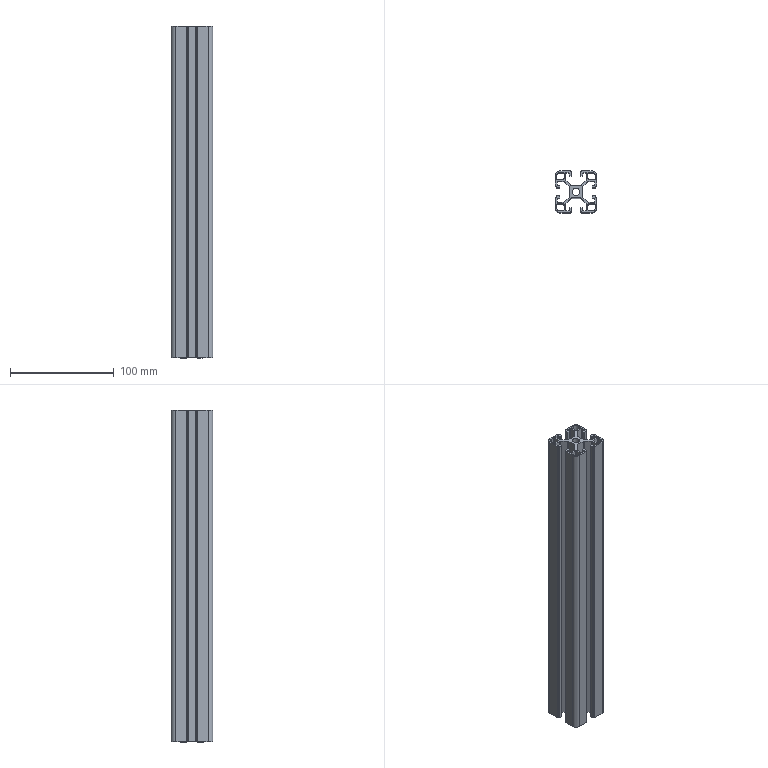Part | STEP file | LE-8-4040-S-OO_LE0314010425 | 1 solid | 188 faces | box 40 x 40 x 320 mm | volume 153040 mm3 | cylinder 94 | plane 94 | commonest cylinder face diameters 0.6 x30 2 x28 4 x16 0.4 x8 6 x4 9 x4